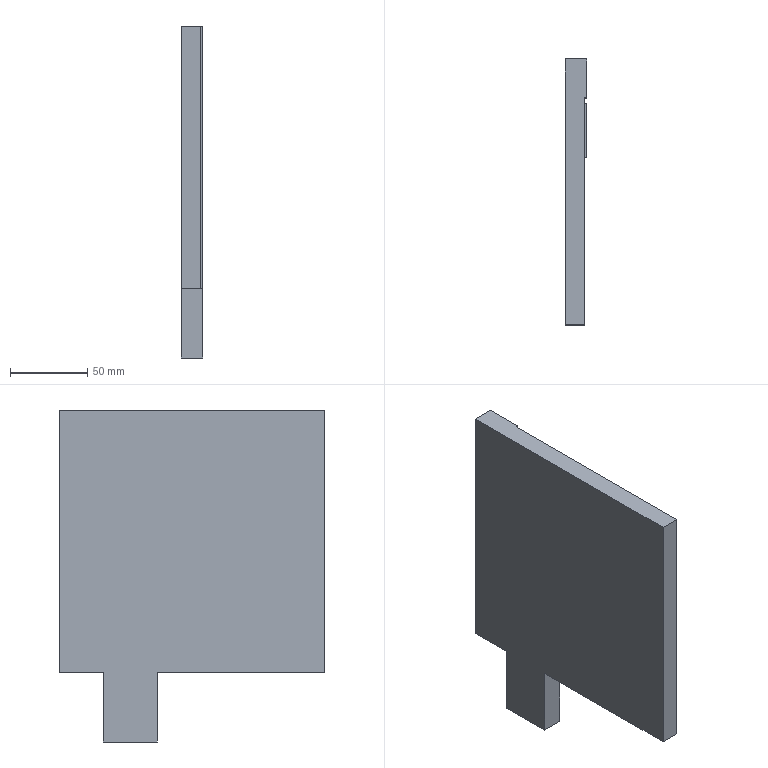Part | SolidWorks | features ICE 2, 3DProfileFeature 1, Extrusion 1, HoleWzd 1 | 1 solid | 14 faces | box 14 x 172 x 215 mm | volume 393925 mm3 | plane 14
STEP:
#1=CARTESIAN_POINT('',(0.,143.5,-85.));
#2=VERTEX_POINT('',#1);
#3=CARTESIAN_POINT('',(12.5,143.5,-85.));
#4=VERTEX_POINT('',#3);
#5=CARTESIAN_POINT('',(14.,143.5,-85.));
#6=DIRECTION('',(1.,0.,0.));
#7=VECTOR('',#6,1000.);
#8=LINE('',#5,#7);
#9=EDGE_CURVE('',#2,#4,#8,.T.);
#10=ORIENTED_EDGE('',*,*,#9,.F.);
#11=CARTESIAN_POINT('',(0.,172.,-85.));
#12=VERTEX_POINT('',#11);
#13=CARTESIAN_POINT('',(0.,0.,-85.));
#14=DIRECTION('',(0.,-1.,0.));
#15=VECTOR('',#14,1000.);
#16=LINE('',#13,#15);
#17=EDGE_CURVE('',#12,#2,#16,.T.);
#18=ORIENTED_EDGE('',*,*,#17,.F.);
#19=CARTESIAN_POINT('',(14.,172.,-85.));
#20=VERTEX_POINT('',#19);
#21=CARTESIAN_POINT('',(0.,172.,-85.));
#22=DIRECTION('',(-1.,0.,0.));
#23=VECTOR('',#22,1000.);
#24=LINE('',#21,#23);
#25=EDGE_CURVE('',#20,#12,#24,.T.);
#26=ORIENTED_EDGE('',*,*,#25,.F.);
#27=CARTESIAN_POINT('',(14.,147.,-85.));
#28=VERTEX_POINT('',#27);
#29=CARTESIAN_POINT('',(14.,172.,-85.));
#30=DIRECTION('',(0.,1.,0.));
#31=VECTOR('',#30,1000.);
#32=LINE('',#29,#31);
#33=EDGE_CURVE('',#28,#20,#32,.T.);
#34=ORIENTED_EDGE('',*,*,#33,.F.);
#35=CARTESIAN_POINT('',(12.5,147.,-85.));
#36=VERTEX_POINT('',#35);
#37=CARTESIAN_POINT('',(14.,147.,-85.));
#38=DIRECTION('',(1.,0.,0.));
#39=VECTOR('',#38,1000.);
#40=LINE('',#37,#39);
#41=EDGE_CURVE('',#36,#28,#40,.T.);
#42=ORIENTED_EDGE('',*,*,#41,.F.);
#43=CARTESIAN_POINT('',(12.5,147.,-85.));
#44=DIRECTION('',(0.,1.,0.));
#45=VECTOR('',#44,1000.);
#46=LINE('',#43,#45);
#47=EDGE_CURVE('',#4,#36,#46,.T.);
#48=ORIENTED_EDGE('',*,*,#47,.F.);
#49=EDGE_LOOP('',(#10,#18,#26,#34,#42,#48));
#50=FACE_OUTER_BOUND('',#49,.T.);
#51=CARTESIAN_POINT('',(0.,0.,-85.));
#52=DIRECTION('',(0.,0.,-1.));
#53=DIRECTION('',(-1.,0.,0.));
#54=AXIS2_PLACEMENT_3D('',#51,#52,#53);
#55=PLANE('',#54);
#56=ADVANCED_FACE('',(#50),#55,.T.);
#57=CARTESIAN_POINT('',(0.,0.,-85.));
#58=VERTEX_POINT('',#57);
#59=CARTESIAN_POINT('',(12.5,0.,-85.));
#60=VERTEX_POINT('',#59);
#61=CARTESIAN_POINT('',(12.5,0.,-85.));
#62=DIRECTION('',(1.,0.,0.));
#63=VECTOR('',#62,1000.);
#64=LINE('',#61,#63);
#65=EDGE_CURVE('',#58,#60,#64,.T.);
#66=ORIENTED_EDGE('',*,*,#65,.T.);
#67=CARTESIAN_POINT('',(12.5,0.,85.));
#68=VERTEX_POINT('',#67);
#69=CARTESIAN_POINT('',(12.5,0.,85.));
#70=DIRECTION('',(0.,0.,-1.));
#71=VECTOR('',#70,1000.);
#72=LINE('',#69,#71);
#73=EDGE_CURVE('',#68,#60,#72,.T.);
#74=ORIENTED_EDGE('',*,*,#73,.F.);
#75=CARTESIAN_POINT('',(0.,0.,85.));
#76=VERTEX_POINT('',#75);
#77=CARTESIAN_POINT('',(12.5,0.,85.));
#78=DIRECTION('',(1.,0.,0.));
#79=VECTOR('',#78,1000.);
#80=LINE('',#77,#79);
#81=EDGE_CURVE('',#76,#68,#80,.T.);
#82=ORIENTED_EDGE('',*,*,#81,.F.);
#83=CARTESIAN_POINT('',(0.,0.,85.));
#84=DIRECTION('',(0.,0.,-1.));
#85=VECTOR('',#84,1000.);
#86=LINE('',#83,#85);
#87=EDGE_CURVE('',#76,#58,#86,.T.);
#88=ORIENTED_EDGE('',*,*,#87,.T.);
#89=EDGE_LOOP('',(#66,#74,#82,#88));
#90=FACE_OUTER_BOUND('',#89,.T.);
#91=CARTESIAN_POINT('',(12.5,0.,85.));
#92=DIRECTION('',(0.,1.,0.));
#93=DIRECTION('',(-1.,0.,0.));
#94=AXIS2_PLACEMENT_3D('',#91,#92,#93);
#95=PLANE('',#94);
#96=ADVANCED_FACE('',(#90),#95,.F.);
#97=CARTESIAN_POINT('',(12.5,108.5,-85.));
#98=VERTEX_POINT('',#97);
#99=CARTESIAN_POINT('',(12.5,147.,-85.));
#100=DIRECTION('',(0.,1.,0.));
#101=VECTOR('',#100,1000.);
#102=LINE('',#99,#101);
#103=EDGE_CURVE('',#60,#98,#102,.T.);
#104=ORIENTED_EDGE('',*,*,#103,.T.);
#105=CARTESIAN_POINT('',(12.5,147.,-85.));
#106=DIRECTION('',(0.,1.,0.));
#107=VECTOR('',#106,1000.);
#108=LINE('',#105,#107);
#109=EDGE_CURVE('',#98,#4,#108,.T.);
#110=ORIENTED_EDGE('',*,*,#109,.T.);
#111=ORIENTED_EDGE('',*,*,#47,.T.);
#112=CARTESIAN_POINT('',(12.5,147.,85.));
#113=VERTEX_POINT('',#112);
#114=CARTESIAN_POINT('',(12.5,147.,85.));
#115=DIRECTION('',(0.,0.,-1.));
#116=VECTOR('',#115,1000.);
#117=LINE('',#114,#116);
#118=EDGE_CURVE('',#113,#36,#117,.T.);
#119=ORIENTED_EDGE('',*,*,#118,.F.);
#120=CARTESIAN_POINT('',(12.5,147.,85.));
#121=DIRECTION('',(0.,1.,0.));
#122=VECTOR('',#121,1000.);
#123=LINE('',#120,#122);
#124=EDGE_CURVE('',#68,#113,#123,.T.);
#125=ORIENTED_EDGE('',*,*,#124,.F.);
#126=ORIENTED_EDGE('',*,*,#73,.T.);
#127=EDGE_LOOP('',(#104,#110,#111,#119,#125,#126));
#128=FACE_OUTER_BOUND('',#127,.T.);
#129=CARTESIAN_POINT('',(12.5,147.,85.));
#130=DIRECTION('',(-1.,0.,0.));
#131=DIRECTION('',(0.,-1.,0.));
#132=AXIS2_PLACEMENT_3D('',#129,#130,#131);
#133=PLANE('',#132);
#134=ADVANCED_FACE('',(#128),#133,.F.);
#135=ORIENTED_EDGE('',*,*,#41,.T.);
#136=CARTESIAN_POINT('',(14.,147.,85.));
#137=VERTEX_POINT('',#136);
#138=CARTESIAN_POINT('',(14.,147.,85.));
#139=DIRECTION('',(0.,0.,-1.));
#140=VECTOR('',#139,1000.);
#141=LINE('',#138,#140);
#142=EDGE_CURVE('',#137,#28,#141,.T.);
#143=ORIENTED_EDGE('',*,*,#142,.F.);
#144=CARTESIAN_POINT('',(14.,147.,85.));
#145=DIRECTION('',(1.,0.,0.));
#146=VECTOR('',#145,1000.);
#147=LINE('',#144,#146);
#148=EDGE_CURVE('',#113,#137,#147,.T.);
#149=ORIENTED_EDGE('',*,*,#148,.F.);
#150=ORIENTED_EDGE('',*,*,#118,.T.);
#151=EDGE_LOOP('',(#135,#143,#149,#150));
#152=FACE_OUTER_BOUND('',#151,.T.);
#153=CARTESIAN_POINT('',(14.,147.,85.));
#154=DIRECTION('',(0.,1.,0.));
#155=DIRECTION('',(0.,0.,1.));
#156=AXIS2_PLACEMENT_3D('',#153,#154,#155);
#157=PLANE('',#156);
#158=ADVANCED_FACE('',(#152),#157,.F.);
#159=ORIENTED_EDGE('',*,*,#33,.T.);
#160=CARTESIAN_POINT('',(14.,172.,85.));
#161=VERTEX_POINT('',#160);
#162=CARTESIAN_POINT('',(14.,172.,85.));
#163=DIRECTION('',(0.,0.,-1.));
#164=VECTOR('',#163,1000.);
#165=LINE('',#162,#164);
#166=EDGE_CURVE('',#161,#20,#165,.T.);
#167=ORIENTED_EDGE('',*,*,#166,.F.);
#168=CARTESIAN_POINT('',(14.,172.,85.));
#169=DIRECTION('',(0.,1.,0.));
#170=VECTOR('',#169,1000.);
#171=LINE('',#168,#170);
#172=EDGE_CURVE('',#137,#161,#171,.T.);
#173=ORIENTED_EDGE('',*,*,#172,.F.);
#174=ORIENTED_EDGE('',*,*,#142,.T.);
#175=EDGE_LOOP('',(#159,#167,#173,#174));
#176=FACE_OUTER_BOUND('',#175,.T.);
#177=CARTESIAN_POINT('',(14.,172.,85.));
#178=DIRECTION('',(-1.,0.,0.));
#179=DIRECTION('',(0.,-1.,0.));
#180=AXIS2_PLACEMENT_3D('',#177,#178,#179);
#181=PLANE('',#180);
#182=ADVANCED_FACE('',(#176),#181,.F.);
#183=ORIENTED_EDGE('',*,*,#25,.T.);
#184=CARTESIAN_POINT('',(0.,172.,85.));
#185=VERTEX_POINT('',#184);
#186=CARTESIAN_POINT('',(0.,172.,85.));
#187=DIRECTION('',(0.,0.,-1.));
#188=VECTOR('',#187,1000.);
#189=LINE('',#186,#188);
#190=EDGE_CURVE('',#185,#12,#189,.T.);
#191=ORIENTED_EDGE('',*,*,#190,.F.);
#192=CARTESIAN_POINT('',(0.,172.,85.));
#193=DIRECTION('',(-1.,0.,0.));
#194=VECTOR('',#193,1000.);
#195=LINE('',#192,#194);
#196=EDGE_CURVE('',#161,#185,#195,.T.);
#197=ORIENTED_EDGE('',*,*,#196,.F.);
#198=ORIENTED_EDGE('',*,*,#166,.T.);
#199=EDGE_LOOP('',(#183,#191,#197,#198));
#200=FACE_OUTER_BOUND('',#199,.T.);
#201=CARTESIAN_POINT('',(0.,172.,85.));
#202=DIRECTION('',(0.,-1.,0.));
#203=DIRECTION('',(0.,0.,-1.));
#204=AXIS2_PLACEMENT_3D('',#201,#202,#203);
#205=PLANE('',#204);
#206=ADVANCED_FACE('',(#200),#205,.F.);
#207=ORIENTED_EDGE('',*,*,#17,.T.);
#208=CARTESIAN_POINT('',(0.,143.5,-130.));
#209=VERTEX_POINT('',#208);
#210=CARTESIAN_POINT('',(0.,143.5,-130.));
#211=DIRECTION('',(0.,0.,1.));
#212=VECTOR('',#211,1000.);
#213=LINE('',#210,#212);
#214=EDGE_CURVE('',#209,#2,#213,.T.);
#215=ORIENTED_EDGE('',*,*,#214,.F.);
#216=CARTESIAN_POINT('',(0.,108.5,-130.));
#217=VERTEX_POINT('',#216);
#218=CARTESIAN_POINT('',(0.,143.5,-130.));
#219=DIRECTION('',(0.,1.,0.));
#220=VECTOR('',#219,1000.);
#221=LINE('',#218,#220);
#222=EDGE_CURVE('',#217,#209,#221,.T.);
#223=ORIENTED_EDGE('',*,*,#222,.F.);
#224=CARTESIAN_POINT('',(0.,108.5,-85.));
#225=VERTEX_POINT('',#224);
#226=CARTESIAN_POINT('',(0.,108.5,-130.));
#227=DIRECTION('',(0.,0.,1.));
#228=VECTOR('',#227,1000.);
#229=LINE('',#226,#228);
#230=EDGE_CURVE('',#217,#225,#229,.T.);
#231=ORIENTED_EDGE('',*,*,#230,.T.);
#232=CARTESIAN_POINT('',(0.,0.,-85.));
#233=DIRECTION('',(0.,-1.,0.));
#234=VECTOR('',#233,1000.);
#235=LINE('',#232,#234);
#236=EDGE_CURVE('',#225,#58,#235,.T.);
#237=ORIENTED_EDGE('',*,*,#236,.T.);
#238=ORIENTED_EDGE('',*,*,#87,.F.);
#239=CARTESIAN_POINT('',(0.,0.,85.));
#240=DIRECTION('',(0.,-1.,0.));
#241=VECTOR('',#240,1000.);
#242=LINE('',#239,#241);
#243=EDGE_CURVE('',#185,#76,#242,.T.);
#244=ORIENTED_EDGE('',*,*,#243,.F.);
#245=ORIENTED_EDGE('',*,*,#190,.T.);
#246=EDGE_LOOP('',(#207,#215,#223,#231,#237,#238,#244,#245));
#247=FACE_OUTER_BOUND('',#246,.T.);
#248=CARTESIAN_POINT('',(0.,0.,85.));
#249=DIRECTION('',(1.,0.,0.));
#250=DIRECTION('',(0.,1.,0.));
#251=AXIS2_PLACEMENT_3D('',#248,#249,#250);
#252=PLANE('',#251);
#253=ADVANCED_FACE('',(#247),#252,.F.);
#254=ORIENTED_EDGE('',*,*,#81,.T.);
#255=ORIENTED_EDGE('',*,*,#124,.T.);
#256=ORIENTED_EDGE('',*,*,#148,.T.);
#257=ORIENTED_EDGE('',*,*,#172,.T.);
#258=ORIENTED_EDGE('',*,*,#196,.T.);
#259=ORIENTED_EDGE('',*,*,#243,.T.);
#260=EDGE_LOOP('',(#254,#255,#256,#257,#258,#259));
#261=FACE_OUTER_BOUND('',#260,.T.);
#262=CARTESIAN_POINT('',(0.,0.,85.));
#263=DIRECTION('',(0.,0.,-1.));
#264=DIRECTION('',(-1.,0.,0.));
#265=AXIS2_PLACEMENT_3D('',#262,#263,#264);
#266=PLANE('',#265);
#267=ADVANCED_FACE('',(#261),#266,.F.);
#268=CARTESIAN_POINT('',(14.,108.5,-85.));
#269=DIRECTION('',(-1.,0.,0.));
#270=VECTOR('',#269,1000.);
#271=LINE('',#268,#270);
#272=EDGE_CURVE('',#98,#225,#271,.T.);
#273=ORIENTED_EDGE('',*,*,#272,.F.);
#274=ORIENTED_EDGE('',*,*,#103,.F.);
#275=ORIENTED_EDGE('',*,*,#65,.F.);
#276=ORIENTED_EDGE('',*,*,#236,.F.);
#277=EDGE_LOOP('',(#273,#274,#275,#276));
#278=FACE_OUTER_BOUND('',#277,.T.);
#279=CARTESIAN_POINT('',(0.,0.,-85.));
#280=DIRECTION('',(0.,0.,-1.));
#281=DIRECTION('',(-1.,0.,0.));
#282=AXIS2_PLACEMENT_3D('',#279,#280,#281);
#283=PLANE('',#282);
#284=ADVANCED_FACE('',(#278),#283,.T.);
#285=CARTESIAN_POINT('',(14.,143.5,-85.));
#286=VERTEX_POINT('',#285);
#287=CARTESIAN_POINT('',(14.,108.5,-85.));
#288=VERTEX_POINT('',#287);
#289=CARTESIAN_POINT('',(14.,143.5,-85.));
#290=DIRECTION('',(0.,-1.,0.));
#291=VECTOR('',#290,1000.);
#292=LINE('',#289,#291);
#293=EDGE_CURVE('',#286,#288,#292,.T.);
#294=ORIENTED_EDGE('',*,*,#293,.T.);
#295=CARTESIAN_POINT('',(14.,108.5,-130.));
#296=VERTEX_POINT('',#295);
#297=CARTESIAN_POINT('',(14.,108.5,-130.));
#298=DIRECTION('',(0.,0.,1.));
#299=VECTOR('',#298,1000.);
#300=LINE('',#297,#299);
#301=EDGE_CURVE('',#296,#288,#300,.T.);
#302=ORIENTED_EDGE('',*,*,#301,.F.);
#303=CARTESIAN_POINT('',(14.,143.5,-130.));
#304=VERTEX_POINT('',#303);
#305=CARTESIAN_POINT('',(14.,143.5,-130.));
#306=DIRECTION('',(0.,-1.,0.));
#307=VECTOR('',#306,1000.);
#308=LINE('',#305,#307);
#309=EDGE_CURVE('',#304,#296,#308,.T.);
#310=ORIENTED_EDGE('',*,*,#309,.F.);
#311=CARTESIAN_POINT('',(14.,143.5,-130.));
#312=DIRECTION('',(0.,0.,1.));
#313=VECTOR('',#312,1000.);
#314=LINE('',#311,#313);
#315=EDGE_CURVE('',#304,#286,#314,.T.);
#316=ORIENTED_EDGE('',*,*,#315,.T.);
#317=EDGE_LOOP('',(#294,#302,#310,#316));
#318=FACE_OUTER_BOUND('',#317,.T.);
#319=CARTESIAN_POINT('',(14.,143.5,-130.));
#320=DIRECTION('',(-1.,0.,0.));
#321=DIRECTION('',(0.,-1.,0.));
#322=AXIS2_PLACEMENT_3D('',#319,#320,#321);
#323=PLANE('',#322);
#324=ADVANCED_FACE('',(#318),#323,.F.);
#325=CARTESIAN_POINT('',(14.,108.5,-85.));
#326=DIRECTION('',(-1.,0.,0.));
#327=VECTOR('',#326,1000.);
#328=LINE('',#325,#327);
#329=EDGE_CURVE('',#288,#98,#328,.T.);
#330=ORIENTED_EDGE('',*,*,#329,.T.);
#331=ORIENTED_EDGE('',*,*,#272,.T.);
#332=ORIENTED_EDGE('',*,*,#230,.F.);
#333=CARTESIAN_POINT('',(14.,108.5,-130.));
#334=DIRECTION('',(-1.,0.,0.));
#335=VECTOR('',#334,1000.);
#336=LINE('',#333,#335);
#337=EDGE_CURVE('',#296,#217,#336,.T.);
#338=ORIENTED_EDGE('',*,*,#337,.F.);
#339=ORIENTED_EDGE('',*,*,#301,.T.);
#340=EDGE_LOOP('',(#330,#331,#332,#338,#339));
#341=FACE_OUTER_BOUND('',#340,.T.);
#342=CARTESIAN_POINT('',(14.,108.5,-130.));
#343=DIRECTION('',(0.,1.,0.));
#344=DIRECTION('',(0.,0.,1.));
#345=AXIS2_PLACEMENT_3D('',#342,#343,#344);
#346=PLANE('',#345);
#347=ADVANCED_FACE('',(#341),#346,.F.);
#348=ORIENTED_EDGE('',*,*,#9,.T.);
#349=CARTESIAN_POINT('',(14.,143.5,-85.));
#350=DIRECTION('',(1.,0.,0.));
#351=VECTOR('',#350,1000.);
#352=LINE('',#349,#351);
#353=EDGE_CURVE('',#4,#286,#352,.T.);
#354=ORIENTED_EDGE('',*,*,#353,.T.);
#355=ORIENTED_EDGE('',*,*,#315,.F.);
#356=CARTESIAN_POINT('',(14.,143.5,-130.));
#357=DIRECTION('',(1.,0.,0.));
#358=VECTOR('',#357,1000.);
#359=LINE('',#356,#358);
#360=EDGE_CURVE('',#209,#304,#359,.T.);
#361=ORIENTED_EDGE('',*,*,#360,.F.);
#362=ORIENTED_EDGE('',*,*,#214,.T.);
#363=EDGE_LOOP('',(#348,#354,#355,#361,#362));
#364=FACE_OUTER_BOUND('',#363,.T.);
#365=CARTESIAN_POINT('',(14.,143.5,-130.));
#366=DIRECTION('',(0.,-1.,0.));
#367=DIRECTION('',(0.,0.,-1.));
#368=AXIS2_PLACEMENT_3D('',#365,#366,#367);
#369=PLANE('',#368);
#370=ADVANCED_FACE('',(#364),#369,.F.);
#371=ORIENTED_EDGE('',*,*,#309,.T.);
#372=ORIENTED_EDGE('',*,*,#337,.T.);
#373=ORIENTED_EDGE('',*,*,#222,.T.);
#374=ORIENTED_EDGE('',*,*,#360,.T.);
#375=EDGE_LOOP('',(#371,#372,#373,#374));
#376=FACE_OUTER_BOUND('',#375,.T.);
#377=CARTESIAN_POINT('',(0.,0.,-130.));
#378=DIRECTION('',(0.,0.,-1.));
#379=DIRECTION('',(-1.,0.,0.));
#380=AXIS2_PLACEMENT_3D('',#377,#378,#379);
#381=PLANE('',#380);
#382=ADVANCED_FACE('',(#376),#381,.T.);
#383=ORIENTED_EDGE('',*,*,#109,.F.);
#384=ORIENTED_EDGE('',*,*,#329,.F.);
#385=ORIENTED_EDGE('',*,*,#293,.F.);
#386=ORIENTED_EDGE('',*,*,#353,.F.);
#387=EDGE_LOOP('',(#383,#384,#385,#386));
#388=FACE_OUTER_BOUND('',#387,.T.);
#389=CARTESIAN_POINT('',(0.,0.,-85.));
#390=DIRECTION('',(0.,0.,-1.));
#391=DIRECTION('',(-1.,0.,0.));
#392=AXIS2_PLACEMENT_3D('',#389,#390,#391);
#393=PLANE('',#392);
#394=ADVANCED_FACE('',(#388),#393,.F.);
#395=CLOSED_SHELL('',(#56,#96,#134,#158,#182,#206,#253,#267,#284,#324,#347,#370,#382,#394));
#396=MANIFOLD_SOLID_BREP('',#395);
#397=CARTESIAN_POINT('',(0.,0.,0.));
#398=DIRECTION('',(0.,0.,1.));
#399=DIRECTION('',(1.,0.,0.));
#400=AXIS2_PLACEMENT_3D('',#397,#398,#399);
#401=(LENGTH_UNIT()NAMED_UNIT(*)SI_UNIT(.MILLI.,.METRE.));
#402=UNCERTAINTY_MEASURE_WITH_UNIT(LENGTH_MEASURE(0.00001),#401,'','');
#403=(NAMED_UNIT(*)PLANE_ANGLE_UNIT()SI_UNIT($,.RADIAN.));
#404=(NAMED_UNIT(*)SI_UNIT($,.STERADIAN.)SOLID_ANGLE_UNIT());
#405=(GEOMETRIC_REPRESENTATION_CONTEXT(3)GLOBAL_UNCERTAINTY_ASSIGNED_CONTEXT((#402))GLOBAL_UNIT_ASSIGNED_CONTEXT((#401,#403,#404))REPRESENTATION_CONTEXT('',''));
#406=ADVANCED_BREP_SHAPE_REPRESENTATION('',(#396,#400),#405);